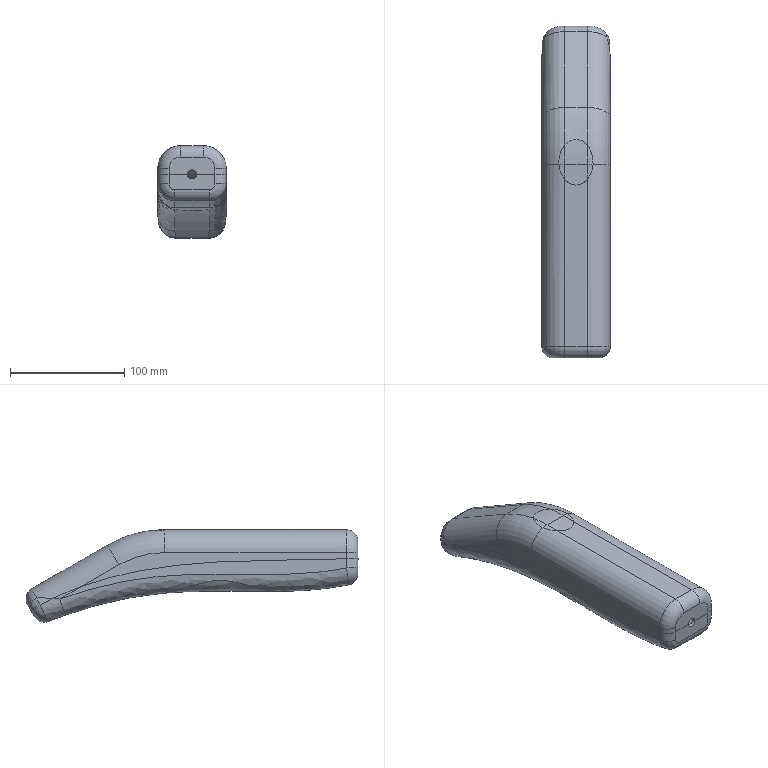Part | SolidWorks | 4 solids | 135 faces | box 60 x 290.622 x 81.047 mm | volume 164282 mm3 | spline 50 | cylinder 43 | plane 26 | torus 16 | commonest cylinder face diameters 14 x8 20 x8 34 x8 40 x8 8 x7 194 x2